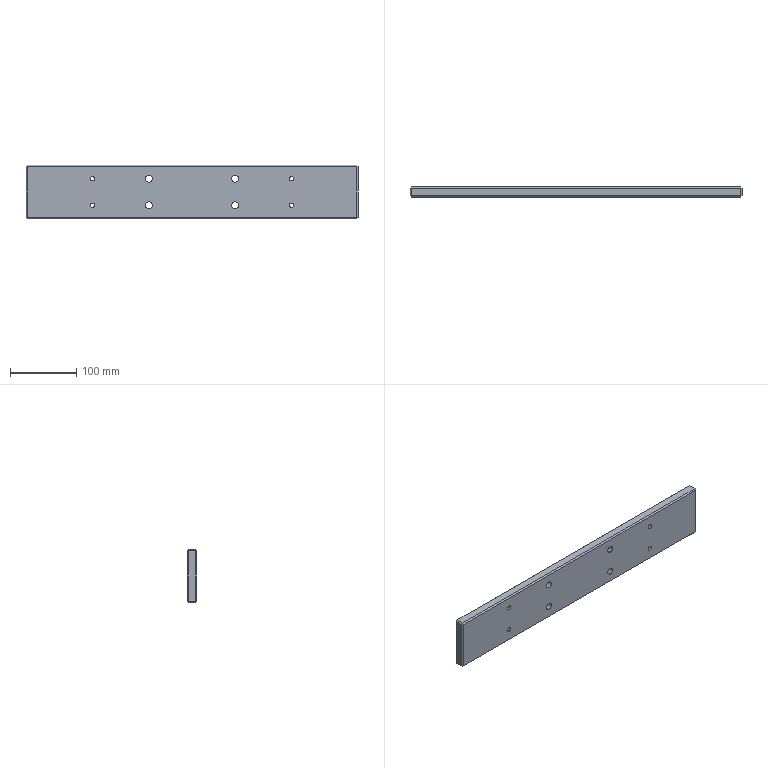Part | SolidWorks | features BaseBody 1 | 1 solid | 42 faces | box 500 x 15 x 80 mm | volume 587908 mm3 | plane 26 | cylinder 16 | commonest cylinder face diameters 6.8 x8 10.5 x8
STEP:
#1=CARTESIAN_POINT('',(-150.,107.,119.721));
#2=VERTEX_POINT('',#1);
#3=CARTESIAN_POINT('',(-150.,107.,126.521));
#4=VERTEX_POINT('',#3);
#5=CARTESIAN_POINT('',(-150.,107.,123.121));
#6=DIRECTION('',(0.,1.,0.));
#7=DIRECTION('',(0.,0.,-1.));
#8=AXIS2_PLACEMENT_3D('',#5,#6,#7);
#9=CIRCLE('',#8,3.4);
#10=EDGE_CURVE('',#2,#4,#9,.T.);
#11=ORIENTED_EDGE('',*,*,#10,.T.);
#12=CARTESIAN_POINT('',(-150.,92.,126.521));
#13=VERTEX_POINT('',#12);
#14=CARTESIAN_POINT('',(-150.,92.,126.521));
#15=DIRECTION('',(0.,-1.,0.));
#16=VECTOR('',#15,1000.);
#17=LINE('',#14,#16);
#18=EDGE_CURVE('',#4,#13,#17,.T.);
#19=ORIENTED_EDGE('',*,*,#18,.T.);
#20=CARTESIAN_POINT('',(-150.,92.,119.721));
#21=VERTEX_POINT('',#20);
#22=CARTESIAN_POINT('',(-150.,92.,123.121));
#23=DIRECTION('',(0.,1.,0.));
#24=DIRECTION('',(0.,0.,-1.));
#25=AXIS2_PLACEMENT_3D('',#22,#23,#24);
#26=CIRCLE('',#25,3.4);
#27=EDGE_CURVE('',#21,#13,#26,.T.);
#28=ORIENTED_EDGE('',*,*,#27,.F.);
#29=CARTESIAN_POINT('',(-150.,92.,119.721));
#30=DIRECTION('',(0.,-1.,0.));
#31=VECTOR('',#30,1000.);
#32=LINE('',#29,#31);
#33=EDGE_CURVE('',#2,#21,#32,.T.);
#34=ORIENTED_EDGE('',*,*,#33,.F.);
#35=EDGE_LOOP('',(#11,#19,#28,#34));
#36=FACE_OUTER_BOUND('',#35,.T.);
#37=CARTESIAN_POINT('',(-150.,92.,123.121));
#38=DIRECTION('',(0.,-1.,0.));
#39=DIRECTION('',(0.,0.,-1.));
#40=AXIS2_PLACEMENT_3D('',#37,#38,#39);
#41=CYLINDRICAL_SURFACE('',#40,3.4);
#42=ADVANCED_FACE('',(#36),#41,.F.);
#43=CARTESIAN_POINT('',(-150.,107.,159.721));
#44=VERTEX_POINT('',#43);
#45=CARTESIAN_POINT('',(-150.,107.,166.521));
#46=VERTEX_POINT('',#45);
#47=CARTESIAN_POINT('',(-150.,107.,163.121));
#48=DIRECTION('',(0.,1.,0.));
#49=DIRECTION('',(0.,0.,-1.));
#50=AXIS2_PLACEMENT_3D('',#47,#48,#49);
#51=CIRCLE('',#50,3.4);
#52=EDGE_CURVE('',#44,#46,#51,.T.);
#53=ORIENTED_EDGE('',*,*,#52,.T.);
#54=CARTESIAN_POINT('',(-150.,92.,166.521));
#55=VERTEX_POINT('',#54);
#56=CARTESIAN_POINT('',(-150.,92.,166.521));
#57=DIRECTION('',(0.,-1.,0.));
#58=VECTOR('',#57,1000.);
#59=LINE('',#56,#58);
#60=EDGE_CURVE('',#46,#55,#59,.T.);
#61=ORIENTED_EDGE('',*,*,#60,.T.);
#62=CARTESIAN_POINT('',(-150.,92.,159.721));
#63=VERTEX_POINT('',#62);
#64=CARTESIAN_POINT('',(-150.,92.,163.121));
#65=DIRECTION('',(0.,1.,0.));
#66=DIRECTION('',(0.,0.,-1.));
#67=AXIS2_PLACEMENT_3D('',#64,#65,#66);
#68=CIRCLE('',#67,3.4);
#69=EDGE_CURVE('',#63,#55,#68,.T.);
#70=ORIENTED_EDGE('',*,*,#69,.F.);
#71=CARTESIAN_POINT('',(-150.,92.,159.721));
#72=DIRECTION('',(0.,-1.,0.));
#73=VECTOR('',#72,1000.);
#74=LINE('',#71,#73);
#75=EDGE_CURVE('',#44,#63,#74,.T.);
#76=ORIENTED_EDGE('',*,*,#75,.F.);
#77=EDGE_LOOP('',(#53,#61,#70,#76));
#78=FACE_OUTER_BOUND('',#77,.T.);
#79=CARTESIAN_POINT('',(-150.,92.,163.121));
#80=DIRECTION('',(0.,-1.,0.));
#81=DIRECTION('',(0.,0.,-1.));
#82=AXIS2_PLACEMENT_3D('',#79,#80,#81);
#83=CYLINDRICAL_SURFACE('',#82,3.4);
#84=ADVANCED_FACE('',(#78),#83,.F.);
#85=CARTESIAN_POINT('',(150.,107.,119.721));
#86=VERTEX_POINT('',#85);
#87=CARTESIAN_POINT('',(150.,107.,126.521));
#88=VERTEX_POINT('',#87);
#89=CARTESIAN_POINT('',(150.,107.,123.121));
#90=DIRECTION('',(0.,1.,0.));
#91=DIRECTION('',(0.,0.,-1.));
#92=AXIS2_PLACEMENT_3D('',#89,#90,#91);
#93=CIRCLE('',#92,3.4);
#94=EDGE_CURVE('',#86,#88,#93,.T.);
#95=ORIENTED_EDGE('',*,*,#94,.T.);
#96=CARTESIAN_POINT('',(150.,92.,126.521));
#97=VERTEX_POINT('',#96);
#98=CARTESIAN_POINT('',(150.,92.,126.521));
#99=DIRECTION('',(0.,-1.,0.));
#100=VECTOR('',#99,1000.);
#101=LINE('',#98,#100);
#102=EDGE_CURVE('',#88,#97,#101,.T.);
#103=ORIENTED_EDGE('',*,*,#102,.T.);
#104=CARTESIAN_POINT('',(150.,92.,119.721));
#105=VERTEX_POINT('',#104);
#106=CARTESIAN_POINT('',(150.,92.,123.121));
#107=DIRECTION('',(0.,1.,0.));
#108=DIRECTION('',(0.,0.,-1.));
#109=AXIS2_PLACEMENT_3D('',#106,#107,#108);
#110=CIRCLE('',#109,3.4);
#111=EDGE_CURVE('',#105,#97,#110,.T.);
#112=ORIENTED_EDGE('',*,*,#111,.F.);
#113=CARTESIAN_POINT('',(150.,92.,119.721));
#114=DIRECTION('',(0.,-1.,0.));
#115=VECTOR('',#114,1000.);
#116=LINE('',#113,#115);
#117=EDGE_CURVE('',#86,#105,#116,.T.);
#118=ORIENTED_EDGE('',*,*,#117,.F.);
#119=EDGE_LOOP('',(#95,#103,#112,#118));
#120=FACE_OUTER_BOUND('',#119,.T.);
#121=CARTESIAN_POINT('',(150.,92.,123.121));
#122=DIRECTION('',(0.,-1.,0.));
#123=DIRECTION('',(0.,0.,-1.));
#124=AXIS2_PLACEMENT_3D('',#121,#122,#123);
#125=CYLINDRICAL_SURFACE('',#124,3.4);
#126=ADVANCED_FACE('',(#120),#125,.F.);
#127=CARTESIAN_POINT('',(150.,107.,159.721));
#128=VERTEX_POINT('',#127);
#129=CARTESIAN_POINT('',(150.,107.,166.521));
#130=VERTEX_POINT('',#129);
#131=CARTESIAN_POINT('',(150.,107.,163.121));
#132=DIRECTION('',(0.,1.,0.));
#133=DIRECTION('',(0.,0.,-1.));
#134=AXIS2_PLACEMENT_3D('',#131,#132,#133);
#135=CIRCLE('',#134,3.4);
#136=EDGE_CURVE('',#128,#130,#135,.T.);
#137=ORIENTED_EDGE('',*,*,#136,.T.);
#138=CARTESIAN_POINT('',(150.,92.,166.521));
#139=VERTEX_POINT('',#138);
#140=CARTESIAN_POINT('',(150.,92.,166.521));
#141=DIRECTION('',(0.,-1.,0.));
#142=VECTOR('',#141,1000.);
#143=LINE('',#140,#142);
#144=EDGE_CURVE('',#130,#139,#143,.T.);
#145=ORIENTED_EDGE('',*,*,#144,.T.);
#146=CARTESIAN_POINT('',(150.,92.,159.721));
#147=VERTEX_POINT('',#146);
#148=CARTESIAN_POINT('',(150.,92.,163.121));
#149=DIRECTION('',(0.,1.,0.));
#150=DIRECTION('',(0.,0.,-1.));
#151=AXIS2_PLACEMENT_3D('',#148,#149,#150);
#152=CIRCLE('',#151,3.4);
#153=EDGE_CURVE('',#147,#139,#152,.T.);
#154=ORIENTED_EDGE('',*,*,#153,.F.);
#155=CARTESIAN_POINT('',(150.,92.,159.721));
#156=DIRECTION('',(0.,-1.,0.));
#157=VECTOR('',#156,1000.);
#158=LINE('',#155,#157);
#159=EDGE_CURVE('',#128,#147,#158,.T.);
#160=ORIENTED_EDGE('',*,*,#159,.F.);
#161=EDGE_LOOP('',(#137,#145,#154,#160));
#162=FACE_OUTER_BOUND('',#161,.T.);
#163=CARTESIAN_POINT('',(150.,92.,163.121));
#164=DIRECTION('',(0.,-1.,0.));
#165=DIRECTION('',(0.,0.,-1.));
#166=AXIS2_PLACEMENT_3D('',#163,#164,#165);
#167=CYLINDRICAL_SURFACE('',#166,3.4);
#168=ADVANCED_FACE('',(#162),#167,.F.);
#169=CARTESIAN_POINT('',(65.,92.,117.871));
#170=VERTEX_POINT('',#169);
#171=CARTESIAN_POINT('',(65.,92.,128.371));
#172=VERTEX_POINT('',#171);
#173=CARTESIAN_POINT('',(65.,92.,123.121));
#174=DIRECTION('',(0.,1.,0.));
#175=DIRECTION('',(0.,0.,1.));
#176=AXIS2_PLACEMENT_3D('',#173,#174,#175);
#177=CIRCLE('',#176,5.25);
#178=EDGE_CURVE('',#170,#172,#177,.T.);
#179=ORIENTED_EDGE('',*,*,#178,.F.);
#180=CARTESIAN_POINT('',(65.,107.,117.871));
#181=VERTEX_POINT('',#180);
#182=CARTESIAN_POINT('',(65.,107.,117.871));
#183=DIRECTION('',(0.,1.,0.));
#184=VECTOR('',#183,1000.);
#185=LINE('',#182,#184);
#186=EDGE_CURVE('',#170,#181,#185,.T.);
#187=ORIENTED_EDGE('',*,*,#186,.T.);
#188=CARTESIAN_POINT('',(65.,107.,128.371));
#189=VERTEX_POINT('',#188);
#190=CARTESIAN_POINT('',(65.,107.,123.121));
#191=DIRECTION('',(0.,1.,0.));
#192=DIRECTION('',(0.,0.,1.));
#193=AXIS2_PLACEMENT_3D('',#190,#191,#192);
#194=CIRCLE('',#193,5.25);
#195=EDGE_CURVE('',#181,#189,#194,.T.);
#196=ORIENTED_EDGE('',*,*,#195,.T.);
#197=CARTESIAN_POINT('',(65.,107.,128.371));
#198=DIRECTION('',(0.,1.,0.));
#199=VECTOR('',#198,1000.);
#200=LINE('',#197,#199);
#201=EDGE_CURVE('',#172,#189,#200,.T.);
#202=ORIENTED_EDGE('',*,*,#201,.F.);
#203=EDGE_LOOP('',(#179,#187,#196,#202));
#204=FACE_OUTER_BOUND('',#203,.T.);
#205=CARTESIAN_POINT('',(65.,107.,123.121));
#206=DIRECTION('',(0.,1.,0.));
#207=DIRECTION('',(0.,0.,1.));
#208=AXIS2_PLACEMENT_3D('',#205,#206,#207);
#209=CYLINDRICAL_SURFACE('',#208,5.25);
#210=ADVANCED_FACE('',(#204),#209,.F.);
#211=CARTESIAN_POINT('',(65.,92.,157.871));
#212=VERTEX_POINT('',#211);
#213=CARTESIAN_POINT('',(65.,92.,168.371));
#214=VERTEX_POINT('',#213);
#215=CARTESIAN_POINT('',(65.,92.,163.121));
#216=DIRECTION('',(0.,1.,0.));
#217=DIRECTION('',(0.,0.,1.));
#218=AXIS2_PLACEMENT_3D('',#215,#216,#217);
#219=CIRCLE('',#218,5.25);
#220=EDGE_CURVE('',#212,#214,#219,.T.);
#221=ORIENTED_EDGE('',*,*,#220,.F.);
#222=CARTESIAN_POINT('',(65.,107.,157.871));
#223=VERTEX_POINT('',#222);
#224=CARTESIAN_POINT('',(65.,107.,157.871));
#225=DIRECTION('',(0.,1.,0.));
#226=VECTOR('',#225,1000.);
#227=LINE('',#224,#226);
#228=EDGE_CURVE('',#212,#223,#227,.T.);
#229=ORIENTED_EDGE('',*,*,#228,.T.);
#230=CARTESIAN_POINT('',(65.,107.,168.371));
#231=VERTEX_POINT('',#230);
#232=CARTESIAN_POINT('',(65.,107.,163.121));
#233=DIRECTION('',(0.,1.,0.));
#234=DIRECTION('',(0.,0.,1.));
#235=AXIS2_PLACEMENT_3D('',#232,#233,#234);
#236=CIRCLE('',#235,5.25);
#237=EDGE_CURVE('',#223,#231,#236,.T.);
#238=ORIENTED_EDGE('',*,*,#237,.T.);
#239=CARTESIAN_POINT('',(65.,107.,168.371));
#240=DIRECTION('',(0.,1.,0.));
#241=VECTOR('',#240,1000.);
#242=LINE('',#239,#241);
#243=EDGE_CURVE('',#214,#231,#242,.T.);
#244=ORIENTED_EDGE('',*,*,#243,.F.);
#245=EDGE_LOOP('',(#221,#229,#238,#244));
#246=FACE_OUTER_BOUND('',#245,.T.);
#247=CARTESIAN_POINT('',(65.,107.,163.121));
#248=DIRECTION('',(0.,1.,0.));
#249=DIRECTION('',(0.,0.,1.));
#250=AXIS2_PLACEMENT_3D('',#247,#248,#249);
#251=CYLINDRICAL_SURFACE('',#250,5.25);
#252=ADVANCED_FACE('',(#246),#251,.F.);
#253=CARTESIAN_POINT('',(-65.,92.,157.871));
#254=VERTEX_POINT('',#253);
#255=CARTESIAN_POINT('',(-65.,92.,168.371));
#256=VERTEX_POINT('',#255);
#257=CARTESIAN_POINT('',(-65.,92.,163.121));
#258=DIRECTION('',(0.,1.,0.));
#259=DIRECTION('',(0.,0.,1.));
#260=AXIS2_PLACEMENT_3D('',#257,#258,#259);
#261=CIRCLE('',#260,5.25);
#262=EDGE_CURVE('',#254,#256,#261,.T.);
#263=ORIENTED_EDGE('',*,*,#262,.F.);
#264=CARTESIAN_POINT('',(-65.,107.,157.871));
#265=VERTEX_POINT('',#264);
#266=CARTESIAN_POINT('',(-65.,107.,157.871));
#267=DIRECTION('',(0.,1.,0.));
#268=VECTOR('',#267,1000.);
#269=LINE('',#266,#268);
#270=EDGE_CURVE('',#254,#265,#269,.T.);
#271=ORIENTED_EDGE('',*,*,#270,.T.);
#272=CARTESIAN_POINT('',(-65.,107.,168.371));
#273=VERTEX_POINT('',#272);
#274=CARTESIAN_POINT('',(-65.,107.,163.121));
#275=DIRECTION('',(0.,1.,0.));
#276=DIRECTION('',(0.,0.,1.));
#277=AXIS2_PLACEMENT_3D('',#274,#275,#276);
#278=CIRCLE('',#277,5.25);
#279=EDGE_CURVE('',#265,#273,#278,.T.);
#280=ORIENTED_EDGE('',*,*,#279,.T.);
#281=CARTESIAN_POINT('',(-65.,107.,168.371));
#282=DIRECTION('',(0.,1.,0.));
#283=VECTOR('',#282,1000.);
#284=LINE('',#281,#283);
#285=EDGE_CURVE('',#256,#273,#284,.T.);
#286=ORIENTED_EDGE('',*,*,#285,.F.);
#287=EDGE_LOOP('',(#263,#271,#280,#286));
#288=FACE_OUTER_BOUND('',#287,.T.);
#289=CARTESIAN_POINT('',(-65.,107.,163.121));
#290=DIRECTION('',(0.,1.,0.));
#291=DIRECTION('',(0.,0.,1.));
#292=AXIS2_PLACEMENT_3D('',#289,#290,#291);
#293=CYLINDRICAL_SURFACE('',#292,5.25);
#294=ADVANCED_FACE('',(#288),#293,.F.);
#295=CARTESIAN_POINT('',(-65.,92.,117.871));
#296=VERTEX_POINT('',#295);
#297=CARTESIAN_POINT('',(-65.,92.,128.371));
#298=VERTEX_POINT('',#297);
#299=CARTESIAN_POINT('',(-65.,92.,123.121));
#300=DIRECTION('',(0.,1.,0.));
#301=DIRECTION('',(0.,0.,1.));
#302=AXIS2_PLACEMENT_3D('',#299,#300,#301);
#303=CIRCLE('',#302,5.25);
#304=EDGE_CURVE('',#296,#298,#303,.T.);
#305=ORIENTED_EDGE('',*,*,#304,.F.);
#306=CARTESIAN_POINT('',(-65.,107.,117.871));
#307=VERTEX_POINT('',#306);
#308=CARTESIAN_POINT('',(-65.,107.,117.871));
#309=DIRECTION('',(0.,1.,0.));
#310=VECTOR('',#309,1000.);
#311=LINE('',#308,#310);
#312=EDGE_CURVE('',#296,#307,#311,.T.);
#313=ORIENTED_EDGE('',*,*,#312,.T.);
#314=CARTESIAN_POINT('',(-65.,107.,128.371));
#315=VERTEX_POINT('',#314);
#316=CARTESIAN_POINT('',(-65.,107.,123.121));
#317=DIRECTION('',(0.,1.,0.));
#318=DIRECTION('',(0.,0.,1.));
#319=AXIS2_PLACEMENT_3D('',#316,#317,#318);
#320=CIRCLE('',#319,5.25);
#321=EDGE_CURVE('',#307,#315,#320,.T.);
#322=ORIENTED_EDGE('',*,*,#321,.T.);
#323=CARTESIAN_POINT('',(-65.,107.,128.371));
#324=DIRECTION('',(0.,1.,0.));
#325=VECTOR('',#324,1000.);
#326=LINE('',#323,#325);
#327=EDGE_CURVE('',#298,#315,#326,.T.);
#328=ORIENTED_EDGE('',*,*,#327,.F.);
#329=EDGE_LOOP('',(#305,#313,#322,#328));
#330=FACE_OUTER_BOUND('',#329,.T.);
#331=CARTESIAN_POINT('',(-65.,107.,123.121));
#332=DIRECTION('',(0.,1.,0.));
#333=DIRECTION('',(0.,0.,1.));
#334=AXIS2_PLACEMENT_3D('',#331,#332,#333);
#335=CYLINDRICAL_SURFACE('',#334,5.25);
#336=ADVANCED_FACE('',(#330),#335,.F.);
#337=CARTESIAN_POINT('',(-248.,107.,181.121));
#338=VERTEX_POINT('',#337);
#339=CARTESIAN_POINT('',(-248.,107.,105.121));
#340=VERTEX_POINT('',#339);
#341=CARTESIAN_POINT('',(-248.,107.,143.121));
#342=DIRECTION('',(0.,0.,-1.));
#343=VECTOR('',#342,1000.);
#344=LINE('',#341,#343);
#345=EDGE_CURVE('',#338,#340,#344,.T.);
#346=ORIENTED_EDGE('',*,*,#345,.F.);
#347=CARTESIAN_POINT('',(248.,107.,181.121));
#348=VERTEX_POINT('',#347);
#349=CARTESIAN_POINT('',(0.,107.,181.121));
#350=DIRECTION('',(-1.,0.,0.));
#351=VECTOR('',#350,1000.);
#352=LINE('',#349,#351);
#353=EDGE_CURVE('',#348,#338,#352,.T.);
#354=ORIENTED_EDGE('',*,*,#353,.F.);
#355=CARTESIAN_POINT('',(248.,107.,105.121));
#356=VERTEX_POINT('',#355);
#357=CARTESIAN_POINT('',(248.,107.,143.121));
#358=DIRECTION('',(0.,0.,1.));
#359=VECTOR('',#358,1000.);
#360=LINE('',#357,#359);
#361=EDGE_CURVE('',#356,#348,#360,.T.);
#362=ORIENTED_EDGE('',*,*,#361,.F.);
#363=CARTESIAN_POINT('',(0.,107.,105.121));
#364=DIRECTION('',(1.,0.,0.));
#365=VECTOR('',#364,1000.);
#366=LINE('',#363,#365);
#367=EDGE_CURVE('',#340,#356,#366,.T.);
#368=ORIENTED_EDGE('',*,*,#367,.F.);
#369=EDGE_LOOP('',(#346,#354,#362,#368));
#370=FACE_OUTER_BOUND('',#369,.T.);
#371=ORIENTED_EDGE('',*,*,#10,.F.);
#372=CARTESIAN_POINT('',(-150.,107.,123.121));
#373=DIRECTION('',(0.,1.,0.));
#374=DIRECTION('',(0.,0.,-1.));
#375=AXIS2_PLACEMENT_3D('',#372,#373,#374);
#376=CIRCLE('',#375,3.4);
#377=EDGE_CURVE('',#4,#2,#376,.T.);
#378=ORIENTED_EDGE('',*,*,#377,.F.);
#379=EDGE_LOOP('',(#371,#378));
#380=FACE_BOUND('',#379,.T.);
#381=ORIENTED_EDGE('',*,*,#52,.F.);
#382=CARTESIAN_POINT('',(-150.,107.,163.121));
#383=DIRECTION('',(0.,1.,0.));
#384=DIRECTION('',(0.,0.,-1.));
#385=AXIS2_PLACEMENT_3D('',#382,#383,#384);
#386=CIRCLE('',#385,3.4);
#387=EDGE_CURVE('',#46,#44,#386,.T.);
#388=ORIENTED_EDGE('',*,*,#387,.F.);
#389=EDGE_LOOP('',(#381,#388));
#390=FACE_BOUND('',#389,.T.);
#391=ORIENTED_EDGE('',*,*,#94,.F.);
#392=CARTESIAN_POINT('',(150.,107.,123.121));
#393=DIRECTION('',(0.,1.,0.));
#394=DIRECTION('',(0.,0.,-1.));
#395=AXIS2_PLACEMENT_3D('',#392,#393,#394);
#396=CIRCLE('',#395,3.4);
#397=EDGE_CURVE('',#88,#86,#396,.T.);
#398=ORIENTED_EDGE('',*,*,#397,.F.);
#399=EDGE_LOOP('',(#391,#398));
#400=FACE_BOUND('',#399,.T.);
#401=ORIENTED_EDGE('',*,*,#136,.F.);
#402=CARTESIAN_POINT('',(150.,107.,163.121));
#403=DIRECTION('',(0.,1.,0.));
#404=DIRECTION('',(0.,0.,-1.));
#405=AXIS2_PLACEMENT_3D('',#402,#403,#404);
#406=CIRCLE('',#405,3.4);
#407=EDGE_CURVE('',#130,#128,#406,.T.);
#408=ORIENTED_EDGE('',*,*,#407,.F.);
#409=EDGE_LOOP('',(#401,#408));
#410=FACE_BOUND('',#409,.T.);
#411=CARTESIAN_POINT('',(65.,107.,123.121));
#412=DIRECTION('',(0.,1.,0.));
#413=DIRECTION('',(0.,0.,1.));
#414=AXIS2_PLACEMENT_3D('',#411,#412,#413);
#415=CIRCLE('',#414,5.25);
#416=EDGE_CURVE('',#189,#181,#415,.T.);
#417=ORIENTED_EDGE('',*,*,#416,.F.);
#418=ORIENTED_EDGE('',*,*,#195,.F.);
#419=EDGE_LOOP('',(#417,#418));
#420=FACE_BOUND('',#419,.T.);
#421=CARTESIAN_POINT('',(65.,107.,163.121));
#422=DIRECTION('',(0.,1.,0.));
#423=DIRECTION('',(0.,0.,1.));
#424=AXIS2_PLACEMENT_3D('',#421,#422,#423);
#425=CIRCLE('',#424,5.25);
#426=EDGE_CURVE('',#231,#223,#425,.T.);
#427=ORIENTED_EDGE('',*,*,#426,.F.);
#428=ORIENTED_EDGE('',*,*,#237,.F.);
#429=EDGE_LOOP('',(#427,#428));
#430=FACE_BOUND('',#429,.T.);
#431=CARTESIAN_POINT('',(-65.,107.,163.121));
#432=DIRECTION('',(0.,1.,0.));
#433=DIRECTION('',(0.,0.,1.));
#434=AXIS2_PLACEMENT_3D('',#431,#432,#433);
#435=CIRCLE('',#434,5.25);
#436=EDGE_CURVE('',#273,#265,#435,.T.);
#437=ORIENTED_EDGE('',*,*,#436,.F.);
#438=ORIENTED_EDGE('',*,*,#279,.F.);
#439=EDGE_LOOP('',(#437,#438));
#440=FACE_BOUND('',#439,.T.);
#441=CARTESIAN_POINT('',(-65.,107.,123.121));
#442=DIRECTION('',(0.,1.,0.));
#443=DIRECTION('',(0.,0.,1.));
#444=AXIS2_PLACEMENT_3D('',#441,#442,#443);
#445=CIRCLE('',#444,5.25);
#446=EDGE_CURVE('',#315,#307,#445,.T.);
#447=ORIENTED_EDGE('',*,*,#446,.F.);
#448=ORIENTED_EDGE('',*,*,#321,.F.);
#449=EDGE_LOOP('',(#447,#448));
#450=FACE_BOUND('',#449,.T.);
#451=CARTESIAN_POINT('',(0.,107.,143.121));
#452=DIRECTION('',(0.,-1.,0.));
#453=DIRECTION('',(0.,0.,-1.));
#454=AXIS2_PLACEMENT_3D('',#451,#452,#453);
#455=PLANE('',#454);
#456=ADVANCED_FACE('',(#370,#380,#390,#400,#410,#420,#430,#440,#450),#455,.F.);
#457=CARTESIAN_POINT('',(-248.,105.,103.121));
#458=VERTEX_POINT('',#457);
#459=CARTESIAN_POINT('',(248.,105.,103.121));
#460=VERTEX_POINT('',#459);
#461=CARTESIAN_POINT('',(-200.,105.,103.121));
#462=DIRECTION('',(1.,0.,0.));
#463=VECTOR('',#462,1000.);
#464=LINE('',#461,#463);
#465=EDGE_CURVE('',#458,#460,#464,.T.);
#466=ORIENTED_EDGE('',*,*,#465,.F.);
#467=CARTESIAN_POINT('',(-248.,105.,103.121));
#468=DIRECTION('',(0.,-0.7071,-0.7071));
#469=VECTOR('',#468,1000.);
#470=LINE('',#467,#469);
#471=EDGE_CURVE('',#340,#458,#470,.T.);
#472=ORIENTED_EDGE('',*,*,#471,.F.);
#473=ORIENTED_EDGE('',*,*,#367,.T.);
#474=CARTESIAN_POINT('',(248.,105.,103.121));
#475=DIRECTION('',(0.,0.7071,0.7071));
#476=VECTOR('',#475,1000.);
#477=LINE('',#474,#476);
#478=EDGE_CURVE('',#460,#356,#477,.T.);
#479=ORIENTED_EDGE('',*,*,#478,.F.);
#480=EDGE_LOOP('',(#466,#472,#473,#479));
#481=FACE_OUTER_BOUND('',#480,.T.);
#482=CARTESIAN_POINT('',(-200.,105.,103.121));
#483=DIRECTION('',(0.,-0.7071,0.7071));
#484=DIRECTION('',(0.,-0.7071,-0.7071));
#485=AXIS2_PLACEMENT_3D('',#482,#483,#484);
#486=PLANE('',#485);
#487=ADVANCED_FACE('',(#481),#486,.F.);
#488=CARTESIAN_POINT('',(-250.,105.,105.121));
#489=VERTEX_POINT('',#488);
#490=CARTESIAN_POINT('',(-250.,105.,105.121));
#491=DIRECTION('',(-0.7071,-0.7071,0.));
#492=VECTOR('',#491,1000.);
#493=LINE('',#490,#492);
#494=EDGE_CURVE('',#340,#489,#493,.T.);
#495=ORIENTED_EDGE('',*,*,#494,.T.);
#496=CARTESIAN_POINT('',(-250.,105.,181.121));
#497=VERTEX_POINT('',#496);
#498=CARTESIAN_POINT('',(-250.,105.,143.121));
#499=DIRECTION('',(0.,0.,1.));
#500=VECTOR('',#499,1000.);
#501=LINE('',#498,#500);
#502=EDGE_CURVE('',#489,#497,#501,.T.);
#503=ORIENTED_EDGE('',*,*,#502,.T.);
#504=CARTESIAN_POINT('',(-250.,105.,181.121));
#505=DIRECTION('',(0.7071,0.7071,0.));
#506=VECTOR('',#505,1000.);
#507=LINE('',#504,#506);
#508=EDGE_CURVE('',#497,#338,#507,.T.);
#509=ORIENTED_EDGE('',*,*,#508,.T.);
#510=ORIENTED_EDGE('',*,*,#345,.T.);
#511=EDGE_LOOP('',(#495,#503,#509,#510));
#512=FACE_OUTER_BOUND('',#511,.T.);
#513=CARTESIAN_POINT('',(-250.,105.,143.121));
#514=DIRECTION('',(-0.7071,0.7071,0.));
#515=DIRECTION('',(-0.7071,-0.7071,0.));
#516=AXIS2_PLACEMENT_3D('',#513,#514,#515);
#517=PLANE('',#516);
#518=ADVANCED_FACE('',(#512),#517,.T.);
#519=ORIENTED_EDGE('',*,*,#353,.T.);
#520=CARTESIAN_POINT('',(-248.,105.,183.121));
#521=VERTEX_POINT('',#520);
#522=CARTESIAN_POINT('',(-248.,105.,183.121));
#523=DIRECTION('',(0.,0.7071,-0.7071));
#524=VECTOR('',#523,1000.);
#525=LINE('',#522,#524);
#526=EDGE_CURVE('',#521,#338,#525,.T.);
#527=ORIENTED_EDGE('',*,*,#526,.F.);
#528=CARTESIAN_POINT('',(248.,105.,183.121));
#529=VERTEX_POINT('',#528);
#530=CARTESIAN_POINT('',(-200.,105.,183.121));
#531=DIRECTION('',(-1.,0.,0.));
#532=VECTOR('',#531,1000.);
#533=LINE('',#530,#532);
#534=EDGE_CURVE('',#529,#521,#533,.T.);
#535=ORIENTED_EDGE('',*,*,#534,.F.);
#536=CARTESIAN_POINT('',(248.,105.,183.121));
#537=DIRECTION('',(0.,-0.7071,0.7071));
#538=VECTOR('',#537,1000.);
#539=LINE('',#536,#538);
#540=EDGE_CURVE('',#348,#529,#539,.T.);
#541=ORIENTED_EDGE('',*,*,#540,.F.);
#542=EDGE_LOOP('',(#519,#527,#535,#541));
#543=FACE_OUTER_BOUND('',#542,.T.);
#544=CARTESIAN_POINT('',(-200.,105.,183.121));
#545=DIRECTION('',(0.,-0.7071,-0.7071));
#546=DIRECTION('',(0.,0.7071,-0.7071));
#547=AXIS2_PLACEMENT_3D('',#544,#545,#546);
#548=PLANE('',#547);
#549=ADVANCED_FACE('',(#543),#548,.F.);
#550=CARTESIAN_POINT('',(250.,105.,105.121));
#551=VERTEX_POINT('',#550);
#552=CARTESIAN_POINT('',(250.,105.,105.121));
#553=DIRECTION('',(-0.7071,0.7071,0.));
#554=VECTOR('',#553,1000.);
#555=LINE('',#552,#554);
#556=EDGE_CURVE('',#551,#356,#555,.T.);
#557=ORIENTED_EDGE('',*,*,#556,.T.);
#558=ORIENTED_EDGE('',*,*,#361,.T.);
#559=CARTESIAN_POINT('',(250.,105.,181.121));
#560=VERTEX_POINT('',#559);
#561=CARTESIAN_POINT('',(250.,105.,181.121));
#562=DIRECTION('',(0.7071,-0.7071,0.));
#563=VECTOR('',#562,1000.);
#564=LINE('',#561,#563);
#565=EDGE_CURVE('',#348,#560,#564,.T.);
#566=ORIENTED_EDGE('',*,*,#565,.T.);
#567=CARTESIAN_POINT('',(250.,105.,143.121));
#568=DIRECTION('',(0.,0.,-1.));
#569=VECTOR('',#568,1000.);
#570=LINE('',#567,#569);
#571=EDGE_CURVE('',#560,#551,#570,.T.);
#572=ORIENTED_EDGE('',*,*,#571,.T.);
#573=EDGE_LOOP('',(#557,#558,#566,#572));
#574=FACE_OUTER_BOUND('',#573,.T.);
#575=CARTESIAN_POINT('',(250.,105.,143.121));
#576=DIRECTION('',(0.7071,0.7071,0.));
#577=DIRECTION('',(-0.7071,0.7071,0.));
#578=AXIS2_PLACEMENT_3D('',#575,#576,#577);
#579=PLANE('',#578);
#580=ADVANCED_FACE('',(#574),#579,.T.);
#581=ORIENTED_EDGE('',*,*,#18,.F.);
#582=ORIENTED_EDGE('',*,*,#377,.T.);
#583=ORIENTED_EDGE('',*,*,#33,.T.);
#584=CARTESIAN_POINT('',(-150.,92.,123.121));
#585=DIRECTION('',(0.,1.,0.));
#586=DIRECTION('',(0.,0.,-1.));
#587=AXIS2_PLACEMENT_3D('',#584,#585,#586);
#588=CIRCLE('',#587,3.4);
#589=EDGE_CURVE('',#13,#21,#588,.T.);
#590=ORIENTED_EDGE('',*,*,#589,.F.);
#591=EDGE_LOOP('',(#581,#582,#583,#590));
#592=FACE_OUTER_BOUND('',#591,.T.);
#593=CARTESIAN_POINT('',(-150.,92.,123.121));
#594=DIRECTION('',(0.,-1.,0.));
#595=DIRECTION('',(0.,0.,-1.));
#596=AXIS2_PLACEMENT_3D('',#593,#594,#595);
#597=CYLINDRICAL_SURFACE('',#596,3.4);
#598=ADVANCED_FACE('',(#592),#597,.F.);
#599=ORIENTED_EDGE('',*,*,#60,.F.);
#600=ORIENTED_EDGE('',*,*,#387,.T.);
#601=ORIENTED_EDGE('',*,*,#75,.T.);
#602=CARTESIAN_POINT('',(-150.,92.,163.121));
#603=DIRECTION('',(0.,1.,0.));
#604=DIRECTION('',(0.,0.,-1.));
#605=AXIS2_PLACEMENT_3D('',#602,#603,#604);
#606=CIRCLE('',#605,3.4);
#607=EDGE_CURVE('',#55,#63,#606,.T.);
#608=ORIENTED_EDGE('',*,*,#607,.F.);
#609=EDGE_LOOP('',(#599,#600,#601,#608));
#610=FACE_OUTER_BOUND('',#609,.T.);
#611=CARTESIAN_POINT('',(-150.,92.,163.121));
#612=DIRECTION('',(0.,-1.,0.));
#613=DIRECTION('',(0.,0.,-1.));
#614=AXIS2_PLACEMENT_3D('',#611,#612,#613);
#615=CYLINDRICAL_SURFACE('',#614,3.4);
#616=ADVANCED_FACE('',(#610),#615,.F.);
#617=ORIENTED_EDGE('',*,*,#102,.F.);
#618=ORIENTED_EDGE('',*,*,#397,.T.);
#619=ORIENTED_EDGE('',*,*,#117,.T.);
#620=CARTESIAN_POINT('',(150.,92.,123.121));
#621=DIRECTION('',(0.,1.,0.));
#622=DIRECTION('',(0.,0.,-1.));
#623=AXIS2_PLACEMENT_3D('',#620,#621,#622);
#624=CIRCLE('',#623,3.4);
#625=EDGE_CURVE('',#97,#105,#624,.T.);
#626=ORIENTED_EDGE('',*,*,#625,.F.);
#627=EDGE_LOOP('',(#617,#618,#619,#626));
#628=FACE_OUTER_BOUND('',#627,.T.);
#629=CARTESIAN_POINT('',(150.,92.,123.121));
#630=DIRECTION('',(0.,-1.,0.));
#631=DIRECTION('',(0.,0.,-1.));
#632=AXIS2_PLACEMENT_3D('',#629,#630,#631);
#633=CYLINDRICAL_SURFACE('',#632,3.4);
#634=ADVANCED_FACE('',(#628),#633,.F.);
#635=ORIENTED_EDGE('',*,*,#144,.F.);
#636=ORIENTED_EDGE('',*,*,#407,.T.);
#637=ORIENTED_EDGE('',*,*,#159,.T.);
#638=CARTESIAN_POINT('',(150.,92.,163.121));
#639=DIRECTION('',(0.,1.,0.));
#640=DIRECTION('',(0.,0.,-1.));
#641=AXIS2_PLACEMENT_3D('',#638,#639,#640);
#642=CIRCLE('',#641,3.4);
#643=EDGE_CURVE('',#139,#147,#642,.T.);
#644=ORIENTED_EDGE('',*,*,#643,.F.);
#645=EDGE_LOOP('',(#635,#636,#637,#644));
#646=FACE_OUTER_BOUND('',#645,.T.);
#647=CARTESIAN_POINT('',(150.,92.,163.121));
#648=DIRECTION('',(0.,-1.,0.));
#649=DIRECTION('',(0.,0.,-1.));
#650=AXIS2_PLACEMENT_3D('',#647,#648,#649);
#651=CYLINDRICAL_SURFACE('',#650,3.4);
#652=ADVANCED_FACE('',(#646),#651,.F.);
#653=ORIENTED_EDGE('',*,*,#186,.F.);
#654=CARTESIAN_POINT('',(65.,92.,123.121));
#655=DIRECTION('',(0.,1.,0.));
#656=DIRECTION('',(0.,0.,1.));
#657=AXIS2_PLACEMENT_3D('',#654,#655,#656);
#658=CIRCLE('',#657,5.25);
#659=EDGE_CURVE('',#172,#170,#658,.T.);
#660=ORIENTED_EDGE('',*,*,#659,.F.);
#661=ORIENTED_EDGE('',*,*,#201,.T.);
#662=ORIENTED_EDGE('',*,*,#416,.T.);
#663=EDGE_LOOP('',(#653,#660,#661,#662));
#664=FACE_OUTER_BOUND('',#663,.T.);
#665=CARTESIAN_POINT('',(65.,107.,123.121));
#666=DIRECTION('',(0.,1.,0.));
#667=DIRECTION('',(0.,0.,1.));
#668=AXIS2_PLACEMENT_3D('',#665,#666,#667);
#669=CYLINDRICAL_SURFACE('',#668,5.25);
#670=ADVANCED_FACE('',(#664),#669,.F.);
#671=ORIENTED_EDGE('',*,*,#228,.F.);
#672=CARTESIAN_POINT('',(65.,92.,163.121));
#673=DIRECTION('',(0.,1.,0.));
#674=DIRECTION('',(0.,0.,1.));
#675=AXIS2_PLACEMENT_3D('',#672,#673,#674);
#676=CIRCLE('',#675,5.25);
#677=EDGE_CURVE('',#214,#212,#676,.T.);
#678=ORIENTED_EDGE('',*,*,#677,.F.);
#679=ORIENTED_EDGE('',*,*,#243,.T.);
#680=ORIENTED_EDGE('',*,*,#426,.T.);
#681=EDGE_LOOP('',(#671,#678,#679,#680));
#682=FACE_OUTER_BOUND('',#681,.T.);
#683=CARTESIAN_POINT('',(65.,107.,163.121));
#684=DIRECTION('',(0.,1.,0.));
#685=DIRECTION('',(0.,0.,1.));
#686=AXIS2_PLACEMENT_3D('',#683,#684,#685);
#687=CYLINDRICAL_SURFACE('',#686,5.25);
#688=ADVANCED_FACE('',(#682),#687,.F.);
#689=ORIENTED_EDGE('',*,*,#270,.F.);
#690=CARTESIAN_POINT('',(-65.,92.,163.121));
#691=DIRECTION('',(0.,1.,0.));
#692=DIRECTION('',(0.,0.,1.));
#693=AXIS2_PLACEMENT_3D('',#690,#691,#692);
#694=CIRCLE('',#693,5.25);
#695=EDGE_CURVE('',#256,#254,#694,.T.);
#696=ORIENTED_EDGE('',*,*,#695,.F.);
#697=ORIENTED_EDGE('',*,*,#285,.T.);
#698=ORIENTED_EDGE('',*,*,#436,.T.);
#699=EDGE_LOOP('',(#689,#696,#697,#698));
#700=FACE_OUTER_BOUND('',#699,.T.);
#701=CARTESIAN_POINT('',(-65.,107.,163.121));
#702=DIRECTION('',(0.,1.,0.));
#703=DIRECTION('',(0.,0.,1.));
#704=AXIS2_PLACEMENT_3D('',#701,#702,#703);
#705=CYLINDRICAL_SURFACE('',#704,5.25);
#706=ADVANCED_FACE('',(#700),#705,.F.);
#707=ORIENTED_EDGE('',*,*,#312,.F.);
#708=CARTESIAN_POINT('',(-65.,92.,123.121));
#709=DIRECTION('',(0.,1.,0.));
#710=DIRECTION('',(0.,0.,1.));
#711=AXIS2_PLACEMENT_3D('',#708,#709,#710);
#712=CIRCLE('',#711,5.25);
#713=EDGE_CURVE('',#298,#296,#712,.T.);
#714=ORIENTED_EDGE('',*,*,#713,.F.);
#715=ORIENTED_EDGE('',*,*,#327,.T.);
#716=ORIENTED_EDGE('',*,*,#446,.T.);
#717=EDGE_LOOP('',(#707,#714,#715,#716));
#718=FACE_OUTER_BOUND('',#717,.T.);
#719=CARTESIAN_POINT('',(-65.,107.,123.121));
#720=DIRECTION('',(0.,1.,0.));
#721=DIRECTION('',(0.,0.,1.));
#722=AXIS2_PLACEMENT_3D('',#719,#720,#721);
#723=CYLINDRICAL_SURFACE('',#722,5.25);
#724=ADVANCED_FACE('',(#718),#723,.F.);
#725=CARTESIAN_POINT('',(248.,105.,103.121));
#726=DIRECTION('',(-0.7071,0.,-0.7071));
#727=VECTOR('',#726,1000.);
#728=LINE('',#725,#727);
#729=EDGE_CURVE('',#551,#460,#728,.T.);
#730=ORIENTED_EDGE('',*,*,#729,.T.);
#731=ORIENTED_EDGE('',*,*,#478,.T.);
#732=ORIENTED_EDGE('',*,*,#556,.F.);
#733=EDGE_LOOP('',(#730,#731,#732));
#734=FACE_OUTER_BOUND('',#733,.T.);
#735=CARTESIAN_POINT('',(248.,105.,103.121));
#736=DIRECTION('',(0.5774,0.5774,-0.5774));
#737=DIRECTION('',(-0.7071,0.,-0.7071));
#738=AXIS2_PLACEMENT_3D('',#735,#736,#737);
#739=PLANE('',#738);
#740=ADVANCED_FACE('',(#734),#739,.T.);
#741=CARTESIAN_POINT('',(-248.,94.,103.121));
#742=VERTEX_POINT('',#741);
#743=CARTESIAN_POINT('',(-248.,92.,103.121));
#744=DIRECTION('',(0.,-1.,0.));
#745=VECTOR('',#744,1000.);
#746=LINE('',#743,#745);
#747=EDGE_CURVE('',#458,#742,#746,.T.);
#748=ORIENTED_EDGE('',*,*,#747,.F.);
#749=ORIENTED_EDGE('',*,*,#465,.T.);
#750=CARTESIAN_POINT('',(248.,94.,103.121));
#751=VERTEX_POINT('',#750);
#752=CARTESIAN_POINT('',(248.,92.,103.121));
#753=DIRECTION('',(0.,1.,0.));
#754=VECTOR('',#753,1000.);
#755=LINE('',#752,#754);
#756=EDGE_CURVE('',#751,#460,#755,.T.);
#757=ORIENTED_EDGE('',*,*,#756,.F.);
#758=CARTESIAN_POINT('',(-200.,94.,103.121));
#759=DIRECTION('',(1.,0.,0.));
#760=VECTOR('',#759,1000.);
#761=LINE('',#758,#760);
#762=EDGE_CURVE('',#742,#751,#761,.T.);
#763=ORIENTED_EDGE('',*,*,#762,.F.);
#764=EDGE_LOOP('',(#748,#749,#757,#763));
#765=FACE_OUTER_BOUND('',#764,.T.);
#766=CARTESIAN_POINT('',(-200.,92.,103.121));
#767=DIRECTION('',(0.,0.,1.));
#768=DIRECTION('',(1.,0.,0.));
#769=AXIS2_PLACEMENT_3D('',#766,#767,#768);
#770=PLANE('',#769);
#771=ADVANCED_FACE('',(#765),#770,.F.);
#772=ORIENTED_EDGE('',*,*,#471,.T.);
#773=CARTESIAN_POINT('',(-248.,105.,103.121));
#774=DIRECTION('',(-0.7071,0.,0.7071));
#775=VECTOR('',#774,1000.);
#776=LINE('',#773,#775);
#777=EDGE_CURVE('',#458,#489,#776,.T.);
#778=ORIENTED_EDGE('',*,*,#777,.T.);
#779=ORIENTED_EDGE('',*,*,#494,.F.);
#780=EDGE_LOOP('',(#772,#778,#779));
#781=FACE_OUTER_BOUND('',#780,.T.);
#782=CARTESIAN_POINT('',(-248.,105.,103.121));
#783=DIRECTION('',(-0.5774,0.5774,-0.5774));
#784=DIRECTION('',(-0.7071,0.,0.7071));
#785=AXIS2_PLACEMENT_3D('',#782,#783,#784);
#786=PLANE('',#785);
#787=ADVANCED_FACE('',(#781),#786,.T.);
#788=CARTESIAN_POINT('',(-250.,94.,105.121));
#789=VERTEX_POINT('',#788);
#790=CARTESIAN_POINT('',(-250.,94.,181.121));
#791=VERTEX_POINT('',#790);
#792=CARTESIAN_POINT('',(-250.,94.,143.121));
#793=DIRECTION('',(0.,0.,1.));
#794=VECTOR('',#793,1000.);
#795=LINE('',#792,#794);
#796=EDGE_CURVE('',#789,#791,#795,.T.);
#797=ORIENTED_EDGE('',*,*,#796,.T.);
#798=CARTESIAN_POINT('',(-250.,107.,181.121));
#799=DIRECTION('',(0.,1.,0.));
#800=VECTOR('',#799,1000.);
#801=LINE('',#798,#800);
#802=EDGE_CURVE('',#791,#497,#801,.T.);
#803=ORIENTED_EDGE('',*,*,#802,.T.);
#804=ORIENTED_EDGE('',*,*,#502,.F.);
#805=CARTESIAN_POINT('',(-250.,107.,105.121));
#806=DIRECTION('',(0.,-1.,0.));
#807=VECTOR('',#806,1000.);
#808=LINE('',#805,#807);
#809=EDGE_CURVE('',#489,#789,#808,.T.);
#810=ORIENTED_EDGE('',*,*,#809,.T.);
#811=EDGE_LOOP('',(#797,#803,#804,#810));
#812=FACE_OUTER_BOUND('',#811,.T.);
#813=CARTESIAN_POINT('',(-250.,107.,143.121));
#814=DIRECTION('',(-1.,0.,0.));
#815=DIRECTION('',(0.,0.,1.));
#816=AXIS2_PLACEMENT_3D('',#813,#814,#815);
#817=PLANE('',#816);
#818=ADVANCED_FACE('',(#812),#817,.T.);
#819=ORIENTED_EDGE('',*,*,#526,.T.);
#820=ORIENTED_EDGE('',*,*,#508,.F.);
#821=CARTESIAN_POINT('',(-249.,105.,182.121));
#822=DIRECTION('',(0.7071,0.,0.7071));
#823=VECTOR('',#822,1000.);
#824=LINE('',#821,#823);
#825=EDGE_CURVE('',#497,#521,#824,.T.);
#826=ORIENTED_EDGE('',*,*,#825,.T.);
#827=EDGE_LOOP('',(#819,#820,#826));
#828=FACE_OUTER_BOUND('',#827,.T.);
#829=CARTESIAN_POINT('',(-248.,107.,181.121));
#830=DIRECTION('',(-0.5774,0.5774,0.5774));
#831=DIRECTION('',(0.7071,0.,0.7071));
#832=AXIS2_PLACEMENT_3D('',#829,#830,#831);
#833=PLANE('',#832);
#834=ADVANCED_FACE('',(#828),#833,.T.);
#835=CARTESIAN_POINT('',(249.,105.,182.121));
#836=DIRECTION('',(0.7071,0.,-0.7071));
#837=VECTOR('',#836,1000.);
#838=LINE('',#835,#837);
#839=EDGE_CURVE('',#529,#560,#838,.T.);
#840=ORIENTED_EDGE('',*,*,#839,.T.);
#841=ORIENTED_EDGE('',*,*,#565,.F.);
#842=ORIENTED_EDGE('',*,*,#540,.T.);
#843=EDGE_LOOP('',(#840,#841,#842));
#844=FACE_OUTER_BOUND('',#843,.T.);
#845=CARTESIAN_POINT('',(248.,107.,181.121));
#846=DIRECTION('',(0.5774,0.5774,0.5774));
#847=DIRECTION('',(0.7071,0.,-0.7071));
#848=AXIS2_PLACEMENT_3D('',#845,#846,#847);
#849=PLANE('',#848);
#850=ADVANCED_FACE('',(#844),#849,.T.);
#851=CARTESIAN_POINT('',(-248.,94.,183.121));
#852=VERTEX_POINT('',#851);
#853=CARTESIAN_POINT('',(-248.,92.,183.121));
#854=DIRECTION('',(0.,1.,0.));
#855=VECTOR('',#854,1000.);
#856=LINE('',#853,#855);
#857=EDGE_CURVE('',#852,#521,#856,.T.);
#858=ORIENTED_EDGE('',*,*,#857,.F.);
#859=CARTESIAN_POINT('',(248.,94.,183.121));
#860=VERTEX_POINT('',#859);
#861=CARTESIAN_POINT('',(-200.,94.,183.121));
#862=DIRECTION('',(-1.,0.,0.));
#863=VECTOR('',#862,1000.);
#864=LINE('',#861,#863);
#865=EDGE_CURVE('',#860,#852,#864,.T.);
#866=ORIENTED_EDGE('',*,*,#865,.F.);
#867=CARTESIAN_POINT('',(248.,92.,183.121));
#868=DIRECTION('',(0.,-1.,0.));
#869=VECTOR('',#868,1000.);
#870=LINE('',#867,#869);
#871=EDGE_CURVE('',#529,#860,#870,.T.);
#872=ORIENTED_EDGE('',*,*,#871,.F.);
#873=ORIENTED_EDGE('',*,*,#534,.T.);
#874=EDGE_LOOP('',(#858,#866,#872,#873));
#875=FACE_OUTER_BOUND('',#874,.T.);
#876=CARTESIAN_POINT('',(-200.,92.,183.121));
#877=DIRECTION('',(0.,0.,-1.));
#878=DIRECTION('',(-1.,0.,0.));
#879=AXIS2_PLACEMENT_3D('',#876,#877,#878);
#880=PLANE('',#879);
#881=ADVANCED_FACE('',(#875),#880,.F.);
#882=CARTESIAN_POINT('',(250.,94.,181.121));
#883=VERTEX_POINT('',#882);
#884=CARTESIAN_POINT('',(250.,107.,181.121));
#885=DIRECTION('',(0.,-1.,0.));
#886=VECTOR('',#885,1000.);
#887=LINE('',#884,#886);
#888=EDGE_CURVE('',#560,#883,#887,.T.);
#889=ORIENTED_EDGE('',*,*,#888,.T.);
#890=CARTESIAN_POINT('',(250.,94.,105.121));
#891=VERTEX_POINT('',#890);
#892=CARTESIAN_POINT('',(250.,94.,143.121));
#893=DIRECTION('',(0.,0.,-1.));
#894=VECTOR('',#893,1000.);
#895=LINE('',#892,#894);
#896=EDGE_CURVE('',#883,#891,#895,.T.);
#897=ORIENTED_EDGE('',*,*,#896,.T.);
#898=CARTESIAN_POINT('',(250.,107.,105.121));
#899=DIRECTION('',(0.,1.,0.));
#900=VECTOR('',#899,1000.);
#901=LINE('',#898,#900);
#902=EDGE_CURVE('',#891,#551,#901,.T.);
#903=ORIENTED_EDGE('',*,*,#902,.T.);
#904=ORIENTED_EDGE('',*,*,#571,.F.);
#905=EDGE_LOOP('',(#889,#897,#903,#904));
#906=FACE_OUTER_BOUND('',#905,.T.);
#907=CARTESIAN_POINT('',(250.,107.,143.121));
#908=DIRECTION('',(1.,0.,0.));
#909=DIRECTION('',(0.,0.,-1.));
#910=AXIS2_PLACEMENT_3D('',#907,#908,#909);
#911=PLANE('',#910);
#912=ADVANCED_FACE('',(#906),#911,.T.);
#913=CARTESIAN_POINT('',(248.,92.,105.121));
#914=VERTEX_POINT('',#913);
#915=CARTESIAN_POINT('',(248.,92.,181.121));
#916=VERTEX_POINT('',#915);
#917=CARTESIAN_POINT('',(248.,92.,143.121));
#918=DIRECTION('',(0.,0.,1.));
#919=VECTOR('',#918,1000.);
#920=LINE('',#917,#919);
#921=EDGE_CURVE('',#914,#916,#920,.T.);
#922=ORIENTED_EDGE('',*,*,#921,.T.);
#923=CARTESIAN_POINT('',(-248.,92.,181.121));
#924=VERTEX_POINT('',#923);
#925=CARTESIAN_POINT('',(0.,92.,181.121));
#926=DIRECTION('',(-1.,0.,0.));
#927=VECTOR('',#926,1000.);
#928=LINE('',#925,#927);
#929=EDGE_CURVE('',#916,#924,#928,.T.);
#930=ORIENTED_EDGE('',*,*,#929,.T.);
#931=CARTESIAN_POINT('',(-248.,92.,105.121));
#932=VERTEX_POINT('',#931);
#933=CARTESIAN_POINT('',(-248.,92.,143.121));
#934=DIRECTION('',(0.,0.,-1.));
#935=VECTOR('',#934,1000.);
#936=LINE('',#933,#935);
#937=EDGE_CURVE('',#924,#932,#936,.T.);
#938=ORIENTED_EDGE('',*,*,#937,.T.);
#939=CARTESIAN_POINT('',(0.,92.,105.121));
#940=DIRECTION('',(1.,0.,0.));
#941=VECTOR('',#940,1000.);
#942=LINE('',#939,#941);
#943=EDGE_CURVE('',#932,#914,#942,.T.);
#944=ORIENTED_EDGE('',*,*,#943,.T.);
#945=EDGE_LOOP('',(#922,#930,#938,#944));
#946=FACE_OUTER_BOUND('',#945,.T.);
#947=ORIENTED_EDGE('',*,*,#27,.T.);
#948=ORIENTED_EDGE('',*,*,#589,.T.);
#949=EDGE_LOOP('',(#947,#948));
#950=FACE_BOUND('',#949,.T.);
#951=ORIENTED_EDGE('',*,*,#69,.T.);
#952=ORIENTED_EDGE('',*,*,#607,.T.);
#953=EDGE_LOOP('',(#951,#952));
#954=FACE_BOUND('',#953,.T.);
#955=ORIENTED_EDGE('',*,*,#111,.T.);
#956=ORIENTED_EDGE('',*,*,#625,.T.);
#957=EDGE_LOOP('',(#955,#956));
#958=FACE_BOUND('',#957,.T.);
#959=ORIENTED_EDGE('',*,*,#153,.T.);
#960=ORIENTED_EDGE('',*,*,#643,.T.);
#961=EDGE_LOOP('',(#959,#960));
#962=FACE_BOUND('',#961,.T.);
#963=ORIENTED_EDGE('',*,*,#659,.T.);
#964=ORIENTED_EDGE('',*,*,#178,.T.);
#965=EDGE_LOOP('',(#963,#964));
#966=FACE_BOUND('',#965,.T.);
#967=ORIENTED_EDGE('',*,*,#677,.T.);
#968=ORIENTED_EDGE('',*,*,#220,.T.);
#969=EDGE_LOOP('',(#967,#968));
#970=FACE_BOUND('',#969,.T.);
#971=ORIENTED_EDGE('',*,*,#695,.T.);
#972=ORIENTED_EDGE('',*,*,#262,.T.);
#973=EDGE_LOOP('',(#971,#972));
#974=FACE_BOUND('',#973,.T.);
#975=ORIENTED_EDGE('',*,*,#713,.T.);
#976=ORIENTED_EDGE('',*,*,#304,.T.);
#977=EDGE_LOOP('',(#975,#976));
#978=FACE_BOUND('',#977,.T.);
#979=CARTESIAN_POINT('',(0.,92.,143.121));
#980=DIRECTION('',(0.,-1.,0.));
#981=DIRECTION('',(0.,0.,-1.));
#982=AXIS2_PLACEMENT_3D('',#979,#980,#981);
#983=PLANE('',#982);
#984=ADVANCED_FACE('',(#946,#950,#954,#958,#962,#966,#970,#974,#978),#983,.T.);
#985=CARTESIAN_POINT('',(250.,94.,105.121));
#986=DIRECTION('',(-0.7071,0.,-0.7071));
#987=VECTOR('',#986,1000.);
#988=LINE('',#985,#987);
#989=EDGE_CURVE('',#891,#751,#988,.T.);
#990=ORIENTED_EDGE('',*,*,#989,.T.);
#991=ORIENTED_EDGE('',*,*,#756,.T.);
#992=ORIENTED_EDGE('',*,*,#729,.F.);
#993=ORIENTED_EDGE('',*,*,#902,.F.);
#994=EDGE_LOOP('',(#990,#991,#992,#993));
#995=FACE_OUTER_BOUND('',#994,.T.);
#996=CARTESIAN_POINT('',(250.,107.,105.121));
#997=DIRECTION('',(0.7071,0.,-0.7071));
#998=DIRECTION('',(-0.7071,0.,-0.7071));
#999=AXIS2_PLACEMENT_3D('',#996,#997,#998);
#1000=PLANE('',#999);
#1001=ADVANCED_FACE('',(#995),#1000,.T.);
#1002=CARTESIAN_POINT('',(-248.,92.,105.121));
#1003=DIRECTION('',(0.,0.7071,-0.7071));
#1004=VECTOR('',#1003,1000.);
#1005=LINE('',#1002,#1004);
#1006=EDGE_CURVE('',#932,#742,#1005,.T.);
#1007=ORIENTED_EDGE('',*,*,#1006,.T.);
#1008=ORIENTED_EDGE('',*,*,#762,.T.);
#1009=CARTESIAN_POINT('',(248.,92.,105.121));
#1010=DIRECTION('',(0.,-0.7071,0.7071));
#1011=VECTOR('',#1010,1000.);
#1012=LINE('',#1009,#1011);
#1013=EDGE_CURVE('',#751,#914,#1012,.T.);
#1014=ORIENTED_EDGE('',*,*,#1013,.T.);
#1015=ORIENTED_EDGE('',*,*,#943,.F.);
#1016=EDGE_LOOP('',(#1007,#1008,#1014,#1015));
#1017=FACE_OUTER_BOUND('',#1016,.T.);
#1018=CARTESIAN_POINT('',(0.,92.,105.121));
#1019=DIRECTION('',(0.,-0.7071,-0.7071));
#1020=DIRECTION('',(0.,0.7071,-0.7071));
#1021=AXIS2_PLACEMENT_3D('',#1018,#1019,#1020);
#1022=PLANE('',#1021);
#1023=ADVANCED_FACE('',(#1017),#1022,.T.);
#1024=CARTESIAN_POINT('',(-250.,94.,105.121));
#1025=DIRECTION('',(-0.7071,0.,0.7071));
#1026=VECTOR('',#1025,1000.);
#1027=LINE('',#1024,#1026);
#1028=EDGE_CURVE('',#742,#789,#1027,.T.);
#1029=ORIENTED_EDGE('',*,*,#1028,.T.);
#1030=ORIENTED_EDGE('',*,*,#809,.F.);
#1031=ORIENTED_EDGE('',*,*,#777,.F.);
#1032=ORIENTED_EDGE('',*,*,#747,.T.);
#1033=EDGE_LOOP('',(#1029,#1030,#1031,#1032));
#1034=FACE_OUTER_BOUND('',#1033,.T.);
#1035=CARTESIAN_POINT('',(-250.,107.,105.121));
#1036=DIRECTION('',(-0.7071,0.,-0.7071));
#1037=DIRECTION('',(-0.7071,0.,0.7071));
#1038=AXIS2_PLACEMENT_3D('',#1035,#1036,#1037);
#1039=PLANE('',#1038);
#1040=ADVANCED_FACE('',(#1034),#1039,.T.);
#1041=ORIENTED_EDGE('',*,*,#825,.F.);
#1042=ORIENTED_EDGE('',*,*,#802,.F.);
#1043=CARTESIAN_POINT('',(-250.,94.,181.121));
#1044=DIRECTION('',(0.7071,0.,0.7071));
#1045=VECTOR('',#1044,1000.);
#1046=LINE('',#1043,#1045);
#1047=EDGE_CURVE('',#791,#852,#1046,.T.);
#1048=ORIENTED_EDGE('',*,*,#1047,.T.);
#1049=ORIENTED_EDGE('',*,*,#857,.T.);
#1050=EDGE_LOOP('',(#1041,#1042,#1048,#1049));
#1051=FACE_OUTER_BOUND('',#1050,.T.);
#1052=CARTESIAN_POINT('',(-250.,107.,181.121));
#1053=DIRECTION('',(-0.7071,0.,0.7071));
#1054=DIRECTION('',(0.7071,0.,0.7071));
#1055=AXIS2_PLACEMENT_3D('',#1052,#1053,#1054);
#1056=PLANE('',#1055);
#1057=ADVANCED_FACE('',(#1051),#1056,.T.);
#1058=ORIENTED_EDGE('',*,*,#796,.F.);
#1059=CARTESIAN_POINT('',(-250.,94.,105.121));
#1060=DIRECTION('',(-0.7071,0.7071,0.));
#1061=VECTOR('',#1060,1000.);
#1062=LINE('',#1059,#1061);
#1063=EDGE_CURVE('',#932,#789,#1062,.T.);
#1064=ORIENTED_EDGE('',*,*,#1063,.F.);
#1065=ORIENTED_EDGE('',*,*,#937,.F.);
#1066=CARTESIAN_POINT('',(-250.,94.,181.121));
#1067=DIRECTION('',(0.7071,-0.7071,0.));
#1068=VECTOR('',#1067,1000.);
#1069=LINE('',#1066,#1068);
#1070=EDGE_CURVE('',#791,#924,#1069,.T.);
#1071=ORIENTED_EDGE('',*,*,#1070,.F.);
#1072=EDGE_LOOP('',(#1058,#1064,#1065,#1071));
#1073=FACE_OUTER_BOUND('',#1072,.T.);
#1074=CARTESIAN_POINT('',(-250.,94.,143.121));
#1075=DIRECTION('',(0.7071,0.7071,0.));
#1076=DIRECTION('',(-0.7071,0.7071,0.));
#1077=AXIS2_PLACEMENT_3D('',#1074,#1075,#1076);
#1078=PLANE('',#1077);
#1079=ADVANCED_FACE('',(#1073),#1078,.F.);
#1080=CARTESIAN_POINT('',(250.,94.,181.121));
#1081=DIRECTION('',(0.7071,0.,-0.7071));
#1082=VECTOR('',#1081,1000.);
#1083=LINE('',#1080,#1082);
#1084=EDGE_CURVE('',#860,#883,#1083,.T.);
#1085=ORIENTED_EDGE('',*,*,#1084,.T.);
#1086=ORIENTED_EDGE('',*,*,#888,.F.);
#1087=ORIENTED_EDGE('',*,*,#839,.F.);
#1088=ORIENTED_EDGE('',*,*,#871,.T.);
#1089=EDGE_LOOP('',(#1085,#1086,#1087,#1088));
#1090=FACE_OUTER_BOUND('',#1089,.T.);
#1091=CARTESIAN_POINT('',(250.,107.,181.121));
#1092=DIRECTION('',(0.7071,0.,0.7071));
#1093=DIRECTION('',(0.7071,0.,-0.7071));
#1094=AXIS2_PLACEMENT_3D('',#1091,#1092,#1093);
#1095=PLANE('',#1094);
#1096=ADVANCED_FACE('',(#1090),#1095,.T.);
#1097=CARTESIAN_POINT('',(-248.,92.,181.121));
#1098=DIRECTION('',(0.,-0.7071,-0.7071));
#1099=VECTOR('',#1098,1000.);
#1100=LINE('',#1097,#1099);
#1101=EDGE_CURVE('',#852,#924,#1100,.T.);
#1102=ORIENTED_EDGE('',*,*,#1101,.T.);
#1103=ORIENTED_EDGE('',*,*,#929,.F.);
#1104=CARTESIAN_POINT('',(248.,92.,181.121));
#1105=DIRECTION('',(0.,0.7071,0.7071));
#1106=VECTOR('',#1105,1000.);
#1107=LINE('',#1104,#1106);
#1108=EDGE_CURVE('',#916,#860,#1107,.T.);
#1109=ORIENTED_EDGE('',*,*,#1108,.T.);
#1110=ORIENTED_EDGE('',*,*,#865,.T.);
#1111=EDGE_LOOP('',(#1102,#1103,#1109,#1110));
#1112=FACE_OUTER_BOUND('',#1111,.T.);
#1113=CARTESIAN_POINT('',(0.,92.,181.121));
#1114=DIRECTION('',(0.,-0.7071,0.7071));
#1115=DIRECTION('',(0.,-0.7071,-0.7071));
#1116=AXIS2_PLACEMENT_3D('',#1113,#1114,#1115);
#1117=PLANE('',#1116);
#1118=ADVANCED_FACE('',(#1112),#1117,.T.);
#1119=ORIENTED_EDGE('',*,*,#921,.F.);
#1120=CARTESIAN_POINT('',(250.,94.,105.121));
#1121=DIRECTION('',(-0.7071,-0.7071,0.));
#1122=VECTOR('',#1121,1000.);
#1123=LINE('',#1120,#1122);
#1124=EDGE_CURVE('',#891,#914,#1123,.T.);
#1125=ORIENTED_EDGE('',*,*,#1124,.F.);
#1126=ORIENTED_EDGE('',*,*,#896,.F.);
#1127=CARTESIAN_POINT('',(250.,94.,181.121));
#1128=DIRECTION('',(0.7071,0.7071,0.));
#1129=VECTOR('',#1128,1000.);
#1130=LINE('',#1127,#1129);
#1131=EDGE_CURVE('',#916,#883,#1130,.T.);
#1132=ORIENTED_EDGE('',*,*,#1131,.F.);
#1133=EDGE_LOOP('',(#1119,#1125,#1126,#1132));
#1134=FACE_OUTER_BOUND('',#1133,.T.);
#1135=CARTESIAN_POINT('',(250.,94.,143.121));
#1136=DIRECTION('',(-0.7071,0.7071,0.));
#1137=DIRECTION('',(-0.7071,-0.7071,0.));
#1138=AXIS2_PLACEMENT_3D('',#1135,#1136,#1137);
#1139=PLANE('',#1138);
#1140=ADVANCED_FACE('',(#1134),#1139,.F.);
#1141=ORIENTED_EDGE('',*,*,#1124,.T.);
#1142=ORIENTED_EDGE('',*,*,#1013,.F.);
#1143=ORIENTED_EDGE('',*,*,#989,.F.);
#1144=EDGE_LOOP('',(#1141,#1142,#1143));
#1145=FACE_OUTER_BOUND('',#1144,.T.);
#1146=CARTESIAN_POINT('',(248.,94.,103.121));
#1147=DIRECTION('',(0.5774,-0.5774,-0.5774));
#1148=DIRECTION('',(-0.7071,0.,-0.7071));
#1149=AXIS2_PLACEMENT_3D('',#1146,#1147,#1148);
#1150=PLANE('',#1149);
#1151=ADVANCED_FACE('',(#1145),#1150,.T.);
#1152=ORIENTED_EDGE('',*,*,#1063,.T.);
#1153=ORIENTED_EDGE('',*,*,#1028,.F.);
#1154=ORIENTED_EDGE('',*,*,#1006,.F.);
#1155=EDGE_LOOP('',(#1152,#1153,#1154));
#1156=FACE_OUTER_BOUND('',#1155,.T.);
#1157=CARTESIAN_POINT('',(-250.,94.,105.121));
#1158=DIRECTION('',(-0.5774,-0.5774,-0.5774));
#1159=DIRECTION('',(-0.7071,0.,0.7071));
#1160=AXIS2_PLACEMENT_3D('',#1157,#1158,#1159);
#1161=PLANE('',#1160);
#1162=ADVANCED_FACE('',(#1156),#1161,.T.);
#1163=ORIENTED_EDGE('',*,*,#1047,.F.);
#1164=ORIENTED_EDGE('',*,*,#1070,.T.);
#1165=ORIENTED_EDGE('',*,*,#1101,.F.);
#1166=EDGE_LOOP('',(#1163,#1164,#1165));
#1167=FACE_OUTER_BOUND('',#1166,.T.);
#1168=CARTESIAN_POINT('',(-248.,94.,183.121));
#1169=DIRECTION('',(-0.5774,-0.5774,0.5774));
#1170=DIRECTION('',(0.7071,0.,0.7071));
#1171=AXIS2_PLACEMENT_3D('',#1168,#1169,#1170);
#1172=PLANE('',#1171);
#1173=ADVANCED_FACE('',(#1167),#1172,.T.);
#1174=ORIENTED_EDGE('',*,*,#1084,.F.);
#1175=ORIENTED_EDGE('',*,*,#1108,.F.);
#1176=ORIENTED_EDGE('',*,*,#1131,.T.);
#1177=EDGE_LOOP('',(#1174,#1175,#1176));
#1178=FACE_OUTER_BOUND('',#1177,.T.);
#1179=CARTESIAN_POINT('',(250.,94.,181.121));
#1180=DIRECTION('',(0.5774,-0.5774,0.5774));
#1181=DIRECTION('',(0.7071,0.,-0.7071));
#1182=AXIS2_PLACEMENT_3D('',#1179,#1180,#1181);
#1183=PLANE('',#1182);
#1184=ADVANCED_FACE('',(#1178),#1183,.T.);
#1185=CLOSED_SHELL('',(#42,#84,#126,#168,#210,#252,#294,#336,#456,#487,#518,#549,#580,#598,#616,#634,#652,#670,#688,#706,#724,#740,#771,#787,#818,#834,#850,#881,#912,#984,#1001,#1023,#1040,#1057,#1079,#1096,#1118,#1140,#1151,#1162,#1173,#1184));
#1186=MANIFOLD_SOLID_BREP('',#1185);
#1187=CARTESIAN_POINT('',(0.,0.,0.));
#1188=DIRECTION('',(0.,0.,1.));
#1189=DIRECTION('',(1.,0.,0.));
#1190=AXIS2_PLACEMENT_3D('',#1187,#1188,#1189);
#1191=(LENGTH_UNIT()NAMED_UNIT(*)SI_UNIT(.MILLI.,.METRE.));
#1192=UNCERTAINTY_MEASURE_WITH_UNIT(LENGTH_MEASURE(0.00001),#1191,'','');
#1193=(NAMED_UNIT(*)PLANE_ANGLE_UNIT()SI_UNIT($,.RADIAN.));
#1194=(NAMED_UNIT(*)SI_UNIT($,.STERADIAN.)SOLID_ANGLE_UNIT());
#1195=(GEOMETRIC_REPRESENTATION_CONTEXT(3)GLOBAL_UNCERTAINTY_ASSIGNED_CONTEXT((#1192))GLOBAL_UNIT_ASSIGNED_CONTEXT((#1191,#1193,#1194))REPRESENTATION_CONTEXT('',''));
#1196=ADVANCED_BREP_SHAPE_REPRESENTATION('',(#1186,#1190),#1195);